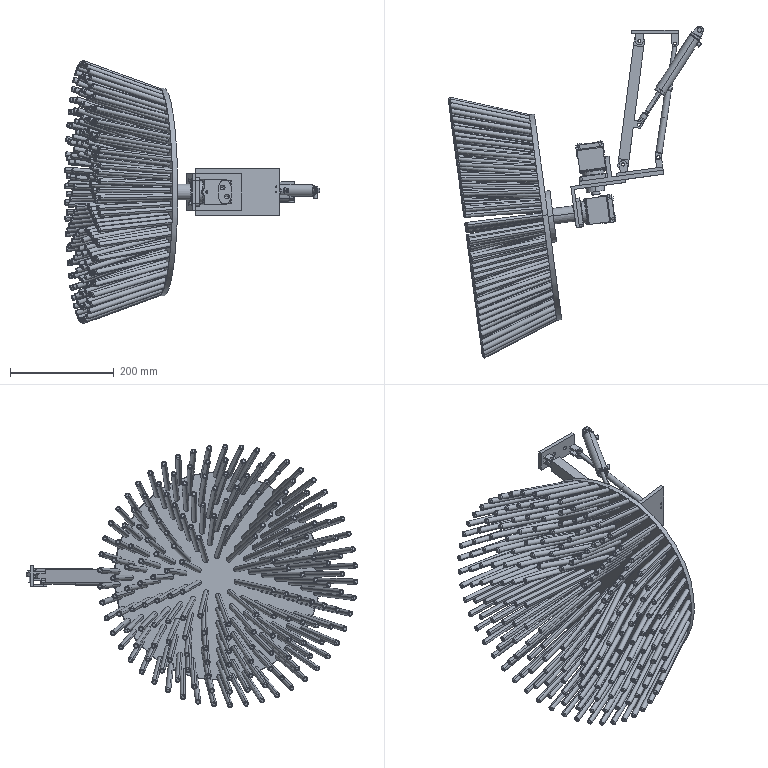Part | SolidWorks | 13 solids | 1814 faces | box 492.003 x 639.962 x 507.373 mm | volume 6091751 mm3 | cylinder 715 | plane 551 | torus 394 | cone 128 | spline 16 | sphere 10 | commonest cylinder face diameters 10 x381 6 x54 16 x40 4 x22 8 x16 9.2 x16